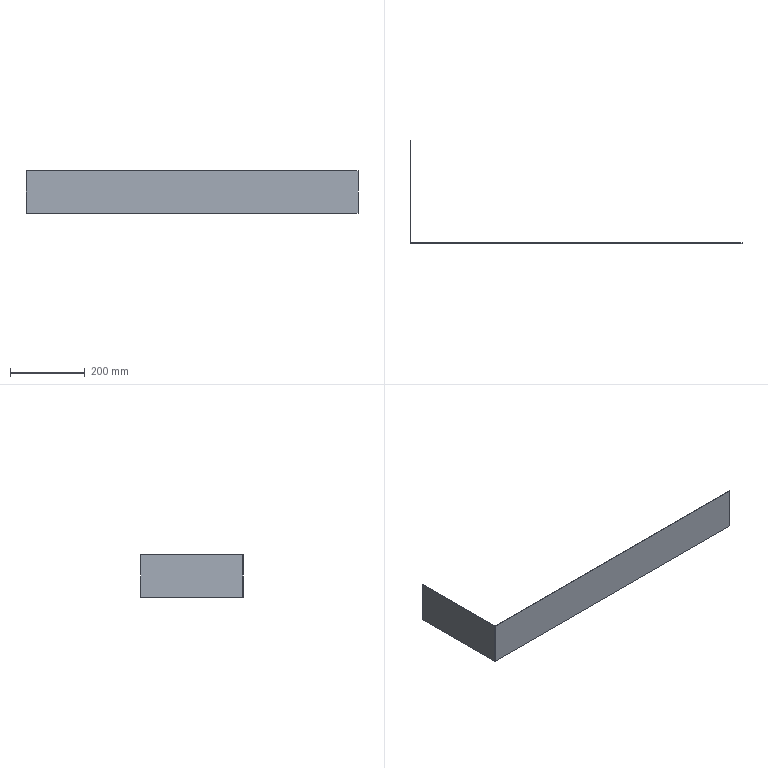Part | STEP file | SX-019-02 | 1 solid | 14 faces | box 890 x 276 x 115 mm | volume 267602 mm3 | plane 12 | cylinder 2 | commonest cylinder face diameters 0.4 x1 4.4 x1
STEP:
#1=CARTESIAN_POINT('',(0.,0.,0.));
#2=DIRECTION('',(0.,0.,1.));
#3=DIRECTION('',(1.,0.,0.));
#4=AXIS2_PLACEMENT_3D('',#1,#2,#3);
#5=CARTESIAN_POINT('',(0.,2.2,115.));
#6=VERTEX_POINT('',#5);
#7=CARTESIAN_POINT('',(2.,2.2,115.));
#8=VERTEX_POINT('',#7);
#9=CARTESIAN_POINT('',(0.,2.2,115.));
#10=DIRECTION('',(1.,0.,0.));
#11=VECTOR('',#10,1.);
#12=LINE('',#9,#11);
#13=CARTESIAN_POINT('',(0.,2.2,115.));
#14=DIRECTION('',(0.,0.,1.));
#15=DIRECTION('',(1.,0.,0.));
#16=AXIS2_PLACEMENT_3D('',#13,#14,#15);
#17=PLANE('',#16);
#18=CARTESIAN_POINT('',(0.,0.));
#19=DIRECTION('',(1.,0.));
#20=VECTOR('',#19,1.);
#21=LINE('',#18,#20);
#22=(GEOMETRIC_REPRESENTATION_CONTEXT(2)PARAMETRIC_REPRESENTATION_CONTEXT()REPRESENTATION_CONTEXT('',''));
#23=DEFINITIONAL_REPRESENTATION('',(#21),#22);
#24=PCURVE('',#17,#23);
#25=CARTESIAN_POINT('',(2.2,2.,115.));
#26=DIRECTION('',(0.,0.,1.));
#27=DIRECTION('',(1.,0.,0.));
#28=AXIS2_PLACEMENT_3D('',#25,#26,#27);
#29=PLANE('',#28);
#30=CARTESIAN_POINT('',(-2.2,0.2));
#31=DIRECTION('',(1.,0.));
#32=VECTOR('',#31,1.);
#33=LINE('',#30,#32);
#34=(GEOMETRIC_REPRESENTATION_CONTEXT(2)PARAMETRIC_REPRESENTATION_CONTEXT()REPRESENTATION_CONTEXT('',''));
#35=DEFINITIONAL_REPRESENTATION('',(#33),#34);
#36=PCURVE('',#29,#35);
#37=SURFACE_CURVE('',#12,(#24,#36),.PCURVE_S1.);
#38=EDGE_CURVE('',#6,#8,#37,.T.);
#39=ORIENTED_EDGE('',*,*,#38,.F.);
#40=CARTESIAN_POINT('',(2.2,0.,115.));
#41=VERTEX_POINT('',#40);
#42=CARTESIAN_POINT('',(2.2,2.2,115.));
#43=DIRECTION('',(0.,0.,1.));
#44=DIRECTION('',(-1.,0.,0.));
#45=AXIS2_PLACEMENT_3D('',#42,#43,#44);
#46=CIRCLE('',#45,2.2);
#47=CARTESIAN_POINT('',(2.2,0.));
#48=DIRECTION('',(-1.,0.));
#49=AXIS2_PLACEMENT_2D('',#47,#48);
#50=CIRCLE('',#49,2.2);
#51=(GEOMETRIC_REPRESENTATION_CONTEXT(2)PARAMETRIC_REPRESENTATION_CONTEXT()REPRESENTATION_CONTEXT('',''));
#52=DEFINITIONAL_REPRESENTATION('',(#50),#51);
#53=PCURVE('',#17,#52);
#54=CARTESIAN_POINT('',(2.2,2.2,115.));
#55=DIRECTION('',(0.,0.,-1.));
#56=DIRECTION('',(-1.,0.,0.));
#57=AXIS2_PLACEMENT_3D('',#54,#55,#56);
#58=CYLINDRICAL_SURFACE('',#57,2.2);
#59=CARTESIAN_POINT('',(6.283,0.));
#60=DIRECTION('',(-1.,0.));
#61=VECTOR('',#60,1.);
#62=LINE('',#59,#61);
#63=(GEOMETRIC_REPRESENTATION_CONTEXT(2)PARAMETRIC_REPRESENTATION_CONTEXT()REPRESENTATION_CONTEXT('',''));
#64=DEFINITIONAL_REPRESENTATION('',(#62),#63);
#65=PCURVE('',#58,#64);
#66=SURFACE_CURVE('',#46,(#53,#65),.PCURVE_S1.);
#67=EDGE_CURVE('',#6,#41,#66,.T.);
#68=ORIENTED_EDGE('',*,*,#67,.T.);
#69=CARTESIAN_POINT('',(2.2,2.,115.));
#70=VERTEX_POINT('',#69);
#71=CARTESIAN_POINT('',(2.2,2.,115.));
#72=DIRECTION('',(0.,-1.,0.));
#73=VECTOR('',#72,1.);
#74=LINE('',#71,#73);
#75=CARTESIAN_POINT('',(2.2,-0.2));
#76=DIRECTION('',(0.,-1.));
#77=VECTOR('',#76,1.);
#78=LINE('',#75,#77);
#79=(GEOMETRIC_REPRESENTATION_CONTEXT(2)PARAMETRIC_REPRESENTATION_CONTEXT()REPRESENTATION_CONTEXT('',''));
#80=DEFINITIONAL_REPRESENTATION('',(#78),#79);
#81=PCURVE('',#17,#80);
#82=CARTESIAN_POINT('',(2.2,2.2,115.));
#83=DIRECTION('',(0.,0.,1.));
#84=DIRECTION('',(1.,0.,0.));
#85=AXIS2_PLACEMENT_3D('',#82,#83,#84);
#86=PLANE('',#85);
#87=CARTESIAN_POINT('',(0.,-0.2));
#88=DIRECTION('',(0.,-1.));
#89=VECTOR('',#88,1.);
#90=LINE('',#87,#89);
#91=(GEOMETRIC_REPRESENTATION_CONTEXT(2)PARAMETRIC_REPRESENTATION_CONTEXT()REPRESENTATION_CONTEXT('',''));
#92=DEFINITIONAL_REPRESENTATION('',(#90),#91);
#93=PCURVE('',#86,#92);
#94=SURFACE_CURVE('',#74,(#81,#93),.PCURVE_S1.);
#95=EDGE_CURVE('',#70,#41,#94,.T.);
#96=ORIENTED_EDGE('',*,*,#95,.F.);
#97=CARTESIAN_POINT('',(2.2,2.2,115.));
#98=DIRECTION('',(0.,0.,1.));
#99=DIRECTION('',(1.,0.,0.));
#100=AXIS2_PLACEMENT_3D('',#97,#98,#99);
#101=CIRCLE('',#100,0.2);
#102=CARTESIAN_POINT('',(2.2,0.));
#103=DIRECTION('',(1.,0.));
#104=AXIS2_PLACEMENT_2D('',#102,#103);
#105=CIRCLE('',#104,0.2);
#106=(GEOMETRIC_REPRESENTATION_CONTEXT(2)PARAMETRIC_REPRESENTATION_CONTEXT()REPRESENTATION_CONTEXT('',''));
#107=DEFINITIONAL_REPRESENTATION('',(#105),#106);
#108=PCURVE('',#17,#107);
#109=CARTESIAN_POINT('',(2.2,2.2,115.));
#110=DIRECTION('',(0.,0.,-1.));
#111=DIRECTION('',(-1.,0.,0.));
#112=AXIS2_PLACEMENT_3D('',#109,#110,#111);
#113=CYLINDRICAL_SURFACE('',#112,0.2);
#114=CARTESIAN_POINT('',(9.425,0.));
#115=DIRECTION('',(-1.,0.));
#116=VECTOR('',#115,1.);
#117=LINE('',#114,#116);
#118=(GEOMETRIC_REPRESENTATION_CONTEXT(2)PARAMETRIC_REPRESENTATION_CONTEXT()REPRESENTATION_CONTEXT('',''));
#119=DEFINITIONAL_REPRESENTATION('',(#117),#118);
#120=PCURVE('',#113,#119);
#121=SURFACE_CURVE('',#101,(#108,#120),.PCURVE_S1.);
#122=EDGE_CURVE('',#8,#70,#121,.T.);
#123=ORIENTED_EDGE('',*,*,#122,.F.);
#124=EDGE_LOOP('',(#39,#68,#96,#123));
#125=FACE_BOUND('',#124,.T.);
#126=ADVANCED_FACE('',(#125),#17,.T.);
#127=CARTESIAN_POINT('',(0.,276.,115.));
#128=VERTEX_POINT('',#127);
#129=CARTESIAN_POINT('',(0.,0.,115.));
#130=DIRECTION('',(0.,-1.,0.));
#131=VECTOR('',#130,1.);
#132=LINE('',#129,#131);
#133=CARTESIAN_POINT('',(-2.2,-2.));
#134=DIRECTION('',(0.,-1.));
#135=VECTOR('',#134,1.);
#136=LINE('',#133,#135);
#137=(GEOMETRIC_REPRESENTATION_CONTEXT(2)PARAMETRIC_REPRESENTATION_CONTEXT()REPRESENTATION_CONTEXT('',''));
#138=DEFINITIONAL_REPRESENTATION('',(#136),#137);
#139=PCURVE('',#29,#138);
#140=CARTESIAN_POINT('',(0.,0.,115.));
#141=DIRECTION('',(1.,0.,0.));
#142=DIRECTION('',(0.,0.,-1.));
#143=AXIS2_PLACEMENT_3D('',#140,#141,#142);
#144=PLANE('',#143);
#145=CARTESIAN_POINT('',(0.,0.));
#146=DIRECTION('',(0.,-1.));
#147=VECTOR('',#146,1.);
#148=LINE('',#145,#147);
#149=(GEOMETRIC_REPRESENTATION_CONTEXT(2)PARAMETRIC_REPRESENTATION_CONTEXT()REPRESENTATION_CONTEXT('',''));
#150=DEFINITIONAL_REPRESENTATION('',(#148),#149);
#151=PCURVE('',#144,#150);
#152=SURFACE_CURVE('',#132,(#139,#151),.PCURVE_S1.);
#153=EDGE_CURVE('',#128,#6,#152,.T.);
#154=ORIENTED_EDGE('',*,*,#153,.T.);
#155=ORIENTED_EDGE('',*,*,#38,.T.);
#156=CARTESIAN_POINT('',(2.,276.,115.));
#157=VERTEX_POINT('',#156);
#158=CARTESIAN_POINT('',(2.,0.,115.));
#159=DIRECTION('',(0.,-1.,0.));
#160=VECTOR('',#159,1.);
#161=LINE('',#158,#160);
#162=CARTESIAN_POINT('',(-0.2,-2.));
#163=DIRECTION('',(0.,-1.));
#164=VECTOR('',#163,1.);
#165=LINE('',#162,#164);
#166=(GEOMETRIC_REPRESENTATION_CONTEXT(2)PARAMETRIC_REPRESENTATION_CONTEXT()REPRESENTATION_CONTEXT('',''));
#167=DEFINITIONAL_REPRESENTATION('',(#165),#166);
#168=PCURVE('',#29,#167);
#169=CARTESIAN_POINT('',(2.,0.,115.));
#170=DIRECTION('',(1.,0.,0.));
#171=DIRECTION('',(0.,0.,-1.));
#172=AXIS2_PLACEMENT_3D('',#169,#170,#171);
#173=PLANE('',#172);
#174=CARTESIAN_POINT('',(0.,0.));
#175=DIRECTION('',(0.,-1.));
#176=VECTOR('',#175,1.);
#177=LINE('',#174,#176);
#178=(GEOMETRIC_REPRESENTATION_CONTEXT(2)PARAMETRIC_REPRESENTATION_CONTEXT()REPRESENTATION_CONTEXT('',''));
#179=DEFINITIONAL_REPRESENTATION('',(#177),#178);
#180=PCURVE('',#173,#179);
#181=SURFACE_CURVE('',#161,(#168,#180),.PCURVE_S1.);
#182=EDGE_CURVE('',#157,#8,#181,.T.);
#183=ORIENTED_EDGE('',*,*,#182,.F.);
#184=CARTESIAN_POINT('',(0.,276.,115.));
#185=DIRECTION('',(1.,0.,0.));
#186=VECTOR('',#185,1.);
#187=LINE('',#184,#186);
#188=CARTESIAN_POINT('',(-2.2,274.));
#189=DIRECTION('',(1.,0.));
#190=VECTOR('',#189,1.);
#191=LINE('',#188,#190);
#192=(GEOMETRIC_REPRESENTATION_CONTEXT(2)PARAMETRIC_REPRESENTATION_CONTEXT()REPRESENTATION_CONTEXT('',''));
#193=DEFINITIONAL_REPRESENTATION('',(#191),#192);
#194=PCURVE('',#29,#193);
#195=CARTESIAN_POINT('',(0.,276.,115.));
#196=DIRECTION('',(0.,1.,0.));
#197=DIRECTION('',(0.,0.,1.));
#198=AXIS2_PLACEMENT_3D('',#195,#196,#197);
#199=PLANE('',#198);
#200=CARTESIAN_POINT('',(0.,0.));
#201=DIRECTION('',(0.,1.));
#202=VECTOR('',#201,1.);
#203=LINE('',#200,#202);
#204=(GEOMETRIC_REPRESENTATION_CONTEXT(2)PARAMETRIC_REPRESENTATION_CONTEXT()REPRESENTATION_CONTEXT('',''));
#205=DEFINITIONAL_REPRESENTATION('',(#203),#204);
#206=PCURVE('',#199,#205);
#207=SURFACE_CURVE('',#187,(#194,#206),.PCURVE_S1.);
#208=EDGE_CURVE('',#128,#157,#207,.T.);
#209=ORIENTED_EDGE('',*,*,#208,.F.);
#210=EDGE_LOOP('',(#154,#155,#183,#209));
#211=FACE_BOUND('',#210,.T.);
#212=ADVANCED_FACE('',(#211),#29,.T.);
#213=CARTESIAN_POINT('',(2.2,0.,0.));
#214=VERTEX_POINT('',#213);
#215=CARTESIAN_POINT('',(2.2,2.,0.));
#216=VERTEX_POINT('',#215);
#217=CARTESIAN_POINT('',(2.2,0.,0.));
#218=DIRECTION('',(0.,1.,0.));
#219=VECTOR('',#218,1.);
#220=LINE('',#217,#219);
#221=CARTESIAN_POINT('',(2.2,0.,0.));
#222=DIRECTION('',(0.,0.,-1.));
#223=DIRECTION('',(-1.,0.,0.));
#224=AXIS2_PLACEMENT_3D('',#221,#222,#223);
#225=PLANE('',#224);
#226=CARTESIAN_POINT('',(0.,0.));
#227=DIRECTION('',(0.,1.));
#228=VECTOR('',#227,1.);
#229=LINE('',#226,#228);
#230=(GEOMETRIC_REPRESENTATION_CONTEXT(2)PARAMETRIC_REPRESENTATION_CONTEXT()REPRESENTATION_CONTEXT('',''));
#231=DEFINITIONAL_REPRESENTATION('',(#229),#230);
#232=PCURVE('',#225,#231);
#233=CARTESIAN_POINT('',(2.,2.2,0.));
#234=DIRECTION('',(0.,0.,-1.));
#235=DIRECTION('',(-1.,0.,0.));
#236=AXIS2_PLACEMENT_3D('',#233,#234,#235);
#237=PLANE('',#236);
#238=CARTESIAN_POINT('',(-0.2,-2.2));
#239=DIRECTION('',(0.,1.));
#240=VECTOR('',#239,1.);
#241=LINE('',#238,#240);
#242=(GEOMETRIC_REPRESENTATION_CONTEXT(2)PARAMETRIC_REPRESENTATION_CONTEXT()REPRESENTATION_CONTEXT('',''));
#243=DEFINITIONAL_REPRESENTATION('',(#241),#242);
#244=PCURVE('',#237,#243);
#245=SURFACE_CURVE('',#220,(#232,#244),.PCURVE_S1.);
#246=EDGE_CURVE('',#214,#216,#245,.T.);
#247=ORIENTED_EDGE('',*,*,#246,.F.);
#248=CARTESIAN_POINT('',(0.,2.2,0.));
#249=VERTEX_POINT('',#248);
#250=CARTESIAN_POINT('',(2.2,2.2,0.));
#251=DIRECTION('',(0.,0.,1.));
#252=DIRECTION('',(-1.,0.,0.));
#253=AXIS2_PLACEMENT_3D('',#250,#251,#252);
#254=CIRCLE('',#253,2.2);
#255=CARTESIAN_POINT('',(2.2,2.2));
#256=CARTESIAN_POINT('',(2.2,-1.611));
#257=CARTESIAN_POINT('',(-1.1,0.2947));
#258=CARTESIAN_POINT('',(-4.4,2.2));
#259=CARTESIAN_POINT('',(-1.1,4.105));
#260=CARTESIAN_POINT('',(2.2,6.011));
#261=CARTESIAN_POINT('',(2.2,2.2));
#262=(BOUNDED_CURVE()B_SPLINE_CURVE(2,(#255,#256,#257,#258,#259,#260,#261),.UNSPECIFIED.,.T.,.F.)B_SPLINE_CURVE_WITH_KNOTS((1,2,2,2,2,1),(-2.094,0.,2.094,4.189,6.283,8.378),.UNSPECIFIED.)CURVE()GEOMETRIC_REPRESENTATION_ITEM()RATIONAL_B_SPLINE_CURVE((1.,0.5,1.,0.5,1.,0.5,1.))REPRESENTATION_ITEM(''));
#263=(GEOMETRIC_REPRESENTATION_CONTEXT(2)PARAMETRIC_REPRESENTATION_CONTEXT()REPRESENTATION_CONTEXT('',''));
#264=DEFINITIONAL_REPRESENTATION('',(#262),#263);
#265=PCURVE('',#225,#264);
#266=CARTESIAN_POINT('',(6.283,115.));
#267=DIRECTION('',(-1.,0.));
#268=VECTOR('',#267,1.);
#269=LINE('',#266,#268);
#270=(GEOMETRIC_REPRESENTATION_CONTEXT(2)PARAMETRIC_REPRESENTATION_CONTEXT()REPRESENTATION_CONTEXT('',''));
#271=DEFINITIONAL_REPRESENTATION('',(#269),#270);
#272=PCURVE('',#58,#271);
#273=SURFACE_CURVE('',#254,(#265,#272),.PCURVE_S1.);
#274=EDGE_CURVE('',#249,#214,#273,.T.);
#275=ORIENTED_EDGE('',*,*,#274,.F.);
#276=CARTESIAN_POINT('',(2.,2.2,0.));
#277=VERTEX_POINT('',#276);
#278=CARTESIAN_POINT('',(2.,2.2,0.));
#279=DIRECTION('',(-1.,0.,0.));
#280=VECTOR('',#279,1.);
#281=LINE('',#278,#280);
#282=CARTESIAN_POINT('',(0.2,2.2));
#283=DIRECTION('',(1.,0.));
#284=VECTOR('',#283,1.);
#285=LINE('',#282,#284);
#286=(GEOMETRIC_REPRESENTATION_CONTEXT(2)PARAMETRIC_REPRESENTATION_CONTEXT()REPRESENTATION_CONTEXT('',''));
#287=DEFINITIONAL_REPRESENTATION('',(#285),#286);
#288=PCURVE('',#225,#287);
#289=CARTESIAN_POINT('',(2.2,2.2,0.));
#290=DIRECTION('',(0.,0.,1.));
#291=DIRECTION('',(1.,0.,0.));
#292=AXIS2_PLACEMENT_3D('',#289,#290,#291);
#293=PLANE('',#292);
#294=CARTESIAN_POINT('',(-0.2,0.));
#295=DIRECTION('',(-1.,0.));
#296=VECTOR('',#295,1.);
#297=LINE('',#294,#296);
#298=(GEOMETRIC_REPRESENTATION_CONTEXT(2)PARAMETRIC_REPRESENTATION_CONTEXT()REPRESENTATION_CONTEXT('',''));
#299=DEFINITIONAL_REPRESENTATION('',(#297),#298);
#300=PCURVE('',#293,#299);
#301=SURFACE_CURVE('',#281,(#288,#300),.PCURVE_S1.);
#302=EDGE_CURVE('',#277,#249,#301,.T.);
#303=ORIENTED_EDGE('',*,*,#302,.F.);
#304=CARTESIAN_POINT('',(2.2,2.2,0.));
#305=DIRECTION('',(0.,0.,1.));
#306=DIRECTION('',(1.,0.,0.));
#307=AXIS2_PLACEMENT_3D('',#304,#305,#306);
#308=CIRCLE('',#307,0.2);
#309=CARTESIAN_POINT('',(-0.2,2.2));
#310=CARTESIAN_POINT('',(-0.2,2.546));
#311=CARTESIAN_POINT('',(0.1,2.373));
#312=CARTESIAN_POINT('',(0.4,2.2));
#313=CARTESIAN_POINT('',(0.1,2.027));
#314=CARTESIAN_POINT('',(-0.2,1.854));
#315=CARTESIAN_POINT('',(-0.2,2.2));
#316=(BOUNDED_CURVE()B_SPLINE_CURVE(2,(#309,#310,#311,#312,#313,#314,#315),.UNSPECIFIED.,.T.,.F.)B_SPLINE_CURVE_WITH_KNOTS((1,2,2,2,2,1),(-2.094,0.,2.094,4.189,6.283,8.378),.UNSPECIFIED.)CURVE()GEOMETRIC_REPRESENTATION_ITEM()RATIONAL_B_SPLINE_CURVE((1.,0.5,1.,0.5,1.,0.5,1.))REPRESENTATION_ITEM(''));
#317=(GEOMETRIC_REPRESENTATION_CONTEXT(2)PARAMETRIC_REPRESENTATION_CONTEXT()REPRESENTATION_CONTEXT('',''));
#318=DEFINITIONAL_REPRESENTATION('',(#316),#317);
#319=PCURVE('',#225,#318);
#320=CARTESIAN_POINT('',(9.425,115.));
#321=DIRECTION('',(-1.,0.));
#322=VECTOR('',#321,1.);
#323=LINE('',#320,#322);
#324=(GEOMETRIC_REPRESENTATION_CONTEXT(2)PARAMETRIC_REPRESENTATION_CONTEXT()REPRESENTATION_CONTEXT('',''));
#325=DEFINITIONAL_REPRESENTATION('',(#323),#324);
#326=PCURVE('',#113,#325);
#327=SURFACE_CURVE('',#308,(#319,#326),.PCURVE_S1.);
#328=EDGE_CURVE('',#277,#216,#327,.T.);
#329=ORIENTED_EDGE('',*,*,#328,.T.);
#330=EDGE_LOOP('',(#247,#275,#303,#329));
#331=FACE_BOUND('',#330,.T.);
#332=ADVANCED_FACE('',(#331),#225,.T.);
#333=CARTESIAN_POINT('',(890.,0.,0.));
#334=VERTEX_POINT('',#333);
#335=CARTESIAN_POINT('',(0.,0.,0.));
#336=DIRECTION('',(1.,0.,0.));
#337=VECTOR('',#336,1.);
#338=LINE('',#335,#337);
#339=CARTESIAN_POINT('',(2.,-2.2));
#340=DIRECTION('',(-1.,0.));
#341=VECTOR('',#340,1.);
#342=LINE('',#339,#341);
#343=(GEOMETRIC_REPRESENTATION_CONTEXT(2)PARAMETRIC_REPRESENTATION_CONTEXT()REPRESENTATION_CONTEXT('',''));
#344=DEFINITIONAL_REPRESENTATION('',(#342),#343);
#345=PCURVE('',#237,#344);
#346=CARTESIAN_POINT('',(0.,0.,115.));
#347=DIRECTION('',(0.,1.,0.));
#348=DIRECTION('',(0.,0.,1.));
#349=AXIS2_PLACEMENT_3D('',#346,#347,#348);
#350=PLANE('',#349);
#351=CARTESIAN_POINT('',(-115.,0.));
#352=DIRECTION('',(0.,1.));
#353=VECTOR('',#352,1.);
#354=LINE('',#351,#353);
#355=(GEOMETRIC_REPRESENTATION_CONTEXT(2)PARAMETRIC_REPRESENTATION_CONTEXT()REPRESENTATION_CONTEXT('',''));
#356=DEFINITIONAL_REPRESENTATION('',(#354),#355);
#357=PCURVE('',#350,#356);
#358=SURFACE_CURVE('',#338,(#345,#357),.PCURVE_S1.);
#359=EDGE_CURVE('',#214,#334,#358,.T.);
#360=ORIENTED_EDGE('',*,*,#359,.F.);
#361=ORIENTED_EDGE('',*,*,#246,.T.);
#362=CARTESIAN_POINT('',(890.,2.,0.));
#363=VERTEX_POINT('',#362);
#364=CARTESIAN_POINT('',(0.,2.,0.));
#365=DIRECTION('',(1.,0.,0.));
#366=VECTOR('',#365,1.);
#367=LINE('',#364,#366);
#368=CARTESIAN_POINT('',(2.,-0.2));
#369=DIRECTION('',(-1.,0.));
#370=VECTOR('',#369,1.);
#371=LINE('',#368,#370);
#372=(GEOMETRIC_REPRESENTATION_CONTEXT(2)PARAMETRIC_REPRESENTATION_CONTEXT()REPRESENTATION_CONTEXT('',''));
#373=DEFINITIONAL_REPRESENTATION('',(#371),#372);
#374=PCURVE('',#237,#373);
#375=CARTESIAN_POINT('',(0.,2.,115.));
#376=DIRECTION('',(0.,1.,0.));
#377=DIRECTION('',(0.,0.,1.));
#378=AXIS2_PLACEMENT_3D('',#375,#376,#377);
#379=PLANE('',#378);
#380=CARTESIAN_POINT('',(-115.,0.));
#381=DIRECTION('',(0.,1.));
#382=VECTOR('',#381,1.);
#383=LINE('',#380,#382);
#384=(GEOMETRIC_REPRESENTATION_CONTEXT(2)PARAMETRIC_REPRESENTATION_CONTEXT()REPRESENTATION_CONTEXT('',''));
#385=DEFINITIONAL_REPRESENTATION('',(#383),#384);
#386=PCURVE('',#379,#385);
#387=SURFACE_CURVE('',#367,(#374,#386),.PCURVE_S1.);
#388=EDGE_CURVE('',#216,#363,#387,.T.);
#389=ORIENTED_EDGE('',*,*,#388,.T.);
#390=CARTESIAN_POINT('',(890.,2.,0.));
#391=DIRECTION('',(0.,-1.,0.));
#392=VECTOR('',#391,1.);
#393=LINE('',#390,#392);
#394=CARTESIAN_POINT('',(-888.,-0.2));
#395=DIRECTION('',(0.,-1.));
#396=VECTOR('',#395,1.);
#397=LINE('',#394,#396);
#398=(GEOMETRIC_REPRESENTATION_CONTEXT(2)PARAMETRIC_REPRESENTATION_CONTEXT()REPRESENTATION_CONTEXT('',''));
#399=DEFINITIONAL_REPRESENTATION('',(#397),#398);
#400=PCURVE('',#237,#399);
#401=CARTESIAN_POINT('',(890.,2.,115.));
#402=DIRECTION('',(1.,0.,0.));
#403=DIRECTION('',(0.,0.,-1.));
#404=AXIS2_PLACEMENT_3D('',#401,#402,#403);
#405=PLANE('',#404);
#406=CARTESIAN_POINT('',(115.,0.));
#407=DIRECTION('',(0.,-1.));
#408=VECTOR('',#407,1.);
#409=LINE('',#406,#408);
#410=(GEOMETRIC_REPRESENTATION_CONTEXT(2)PARAMETRIC_REPRESENTATION_CONTEXT()REPRESENTATION_CONTEXT('',''));
#411=DEFINITIONAL_REPRESENTATION('',(#409),#410);
#412=PCURVE('',#405,#411);
#413=SURFACE_CURVE('',#393,(#400,#412),.PCURVE_S1.);
#414=EDGE_CURVE('',#363,#334,#413,.T.);
#415=ORIENTED_EDGE('',*,*,#414,.T.);
#416=EDGE_LOOP('',(#360,#361,#389,#415));
#417=FACE_BOUND('',#416,.T.);
#418=ADVANCED_FACE('',(#417),#237,.T.);
#419=ORIENTED_EDGE('',*,*,#359,.T.);
#420=CARTESIAN_POINT('',(890.,0.,115.));
#421=VERTEX_POINT('',#420);
#422=CARTESIAN_POINT('',(890.,0.,115.));
#423=DIRECTION('',(0.,0.,-1.));
#424=VECTOR('',#423,1.);
#425=LINE('',#422,#424);
#426=CARTESIAN_POINT('',(0.,890.));
#427=DIRECTION('',(-1.,0.));
#428=VECTOR('',#427,1.);
#429=LINE('',#426,#428);
#430=(GEOMETRIC_REPRESENTATION_CONTEXT(2)PARAMETRIC_REPRESENTATION_CONTEXT()REPRESENTATION_CONTEXT('',''));
#431=DEFINITIONAL_REPRESENTATION('',(#429),#430);
#432=PCURVE('',#350,#431);
#433=CARTESIAN_POINT('',(0.,-2.));
#434=DIRECTION('',(1.,0.));
#435=VECTOR('',#434,1.);
#436=LINE('',#433,#435);
#437=(GEOMETRIC_REPRESENTATION_CONTEXT(2)PARAMETRIC_REPRESENTATION_CONTEXT()REPRESENTATION_CONTEXT('',''));
#438=DEFINITIONAL_REPRESENTATION('',(#436),#437);
#439=PCURVE('',#405,#438);
#440=SURFACE_CURVE('',#425,(#432,#439),.PCURVE_S1.);
#441=EDGE_CURVE('',#421,#334,#440,.T.);
#442=ORIENTED_EDGE('',*,*,#441,.F.);
#443=CARTESIAN_POINT('',(0.,0.,115.));
#444=DIRECTION('',(1.,0.,0.));
#445=VECTOR('',#444,1.);
#446=LINE('',#443,#445);
#447=CARTESIAN_POINT('',(0.,0.));
#448=DIRECTION('',(0.,1.));
#449=VECTOR('',#448,1.);
#450=LINE('',#447,#449);
#451=(GEOMETRIC_REPRESENTATION_CONTEXT(2)PARAMETRIC_REPRESENTATION_CONTEXT()REPRESENTATION_CONTEXT('',''));
#452=DEFINITIONAL_REPRESENTATION('',(#450),#451);
#453=PCURVE('',#350,#452);
#454=CARTESIAN_POINT('',(-2.2,-2.2));
#455=DIRECTION('',(1.,0.));
#456=VECTOR('',#455,1.);
#457=LINE('',#454,#456);
#458=(GEOMETRIC_REPRESENTATION_CONTEXT(2)PARAMETRIC_REPRESENTATION_CONTEXT()REPRESENTATION_CONTEXT('',''));
#459=DEFINITIONAL_REPRESENTATION('',(#457),#458);
#460=PCURVE('',#86,#459);
#461=SURFACE_CURVE('',#446,(#453,#460),.PCURVE_S1.);
#462=EDGE_CURVE('',#41,#421,#461,.T.);
#463=ORIENTED_EDGE('',*,*,#462,.F.);
#464=CARTESIAN_POINT('',(2.2,0.,115.));
#465=DIRECTION('',(0.,0.,-1.));
#466=VECTOR('',#465,1.);
#467=LINE('',#464,#466);
#468=CARTESIAN_POINT('',(0.,2.2));
#469=DIRECTION('',(-1.,0.));
#470=VECTOR('',#469,1.);
#471=LINE('',#468,#470);
#472=(GEOMETRIC_REPRESENTATION_CONTEXT(2)PARAMETRIC_REPRESENTATION_CONTEXT()REPRESENTATION_CONTEXT('',''));
#473=DEFINITIONAL_REPRESENTATION('',(#471),#472);
#474=PCURVE('',#350,#473);
#475=CARTESIAN_POINT('',(4.712,0.));
#476=DIRECTION('',(0.,1.));
#477=VECTOR('',#476,1.);
#478=LINE('',#475,#477);
#479=(GEOMETRIC_REPRESENTATION_CONTEXT(2)PARAMETRIC_REPRESENTATION_CONTEXT()REPRESENTATION_CONTEXT('',''));
#480=DEFINITIONAL_REPRESENTATION('',(#478),#479);
#481=PCURVE('',#58,#480);
#482=SURFACE_CURVE('',#467,(#474,#481),.PCURVE_S1.);
#483=EDGE_CURVE('',#41,#214,#482,.T.);
#484=ORIENTED_EDGE('',*,*,#483,.T.);
#485=EDGE_LOOP('',(#419,#442,#463,#484));
#486=FACE_BOUND('',#485,.T.);
#487=ADVANCED_FACE('',(#486),#350,.F.);
#488=ORIENTED_EDGE('',*,*,#414,.F.);
#489=CARTESIAN_POINT('',(890.,2.,115.));
#490=VERTEX_POINT('',#489);
#491=CARTESIAN_POINT('',(890.,2.,115.));
#492=DIRECTION('',(0.,0.,-1.));
#493=VECTOR('',#492,1.);
#494=LINE('',#491,#493);
#495=CARTESIAN_POINT('',(0.,0.));
#496=DIRECTION('',(1.,0.));
#497=VECTOR('',#496,1.);
#498=LINE('',#495,#497);
#499=(GEOMETRIC_REPRESENTATION_CONTEXT(2)PARAMETRIC_REPRESENTATION_CONTEXT()REPRESENTATION_CONTEXT('',''));
#500=DEFINITIONAL_REPRESENTATION('',(#498),#499);
#501=PCURVE('',#405,#500);
#502=CARTESIAN_POINT('',(0.,890.));
#503=DIRECTION('',(-1.,0.));
#504=VECTOR('',#503,1.);
#505=LINE('',#502,#504);
#506=(GEOMETRIC_REPRESENTATION_CONTEXT(2)PARAMETRIC_REPRESENTATION_CONTEXT()REPRESENTATION_CONTEXT('',''));
#507=DEFINITIONAL_REPRESENTATION('',(#505),#506);
#508=PCURVE('',#379,#507);
#509=SURFACE_CURVE('',#494,(#501,#508),.PCURVE_S1.);
#510=EDGE_CURVE('',#490,#363,#509,.T.);
#511=ORIENTED_EDGE('',*,*,#510,.F.);
#512=CARTESIAN_POINT('',(890.,2.,115.));
#513=DIRECTION('',(0.,-1.,0.));
#514=VECTOR('',#513,1.);
#515=LINE('',#512,#514);
#516=CARTESIAN_POINT('',(0.,0.));
#517=DIRECTION('',(0.,-1.));
#518=VECTOR('',#517,1.);
#519=LINE('',#516,#518);
#520=(GEOMETRIC_REPRESENTATION_CONTEXT(2)PARAMETRIC_REPRESENTATION_CONTEXT()REPRESENTATION_CONTEXT('',''));
#521=DEFINITIONAL_REPRESENTATION('',(#519),#520);
#522=PCURVE('',#405,#521);
#523=CARTESIAN_POINT('',(887.8,-0.2));
#524=DIRECTION('',(0.,-1.));
#525=VECTOR('',#524,1.);
#526=LINE('',#523,#525);
#527=(GEOMETRIC_REPRESENTATION_CONTEXT(2)PARAMETRIC_REPRESENTATION_CONTEXT()REPRESENTATION_CONTEXT('',''));
#528=DEFINITIONAL_REPRESENTATION('',(#526),#527);
#529=PCURVE('',#86,#528);
#530=SURFACE_CURVE('',#515,(#522,#529),.PCURVE_S1.);
#531=EDGE_CURVE('',#490,#421,#530,.T.);
#532=ORIENTED_EDGE('',*,*,#531,.T.);
#533=ORIENTED_EDGE('',*,*,#441,.T.);
#534=EDGE_LOOP('',(#488,#511,#532,#533));
#535=FACE_BOUND('',#534,.T.);
#536=ADVANCED_FACE('',(#535),#405,.T.);
#537=ORIENTED_EDGE('',*,*,#388,.F.);
#538=CARTESIAN_POINT('',(2.2,2.,115.));
#539=DIRECTION('',(0.,0.,-1.));
#540=VECTOR('',#539,1.);
#541=LINE('',#538,#540);
#542=CARTESIAN_POINT('',(0.,2.2));
#543=DIRECTION('',(-1.,0.));
#544=VECTOR('',#543,1.);
#545=LINE('',#542,#544);
#546=(GEOMETRIC_REPRESENTATION_CONTEXT(2)PARAMETRIC_REPRESENTATION_CONTEXT()REPRESENTATION_CONTEXT('',''));
#547=DEFINITIONAL_REPRESENTATION('',(#545),#546);
#548=PCURVE('',#379,#547);
#549=CARTESIAN_POINT('',(4.712,0.));
#550=DIRECTION('',(0.,1.));
#551=VECTOR('',#550,1.);
#552=LINE('',#549,#551);
#553=(GEOMETRIC_REPRESENTATION_CONTEXT(2)PARAMETRIC_REPRESENTATION_CONTEXT()REPRESENTATION_CONTEXT('',''));
#554=DEFINITIONAL_REPRESENTATION('',(#552),#553);
#555=PCURVE('',#113,#554);
#556=SURFACE_CURVE('',#541,(#548,#555),.PCURVE_S1.);
#557=EDGE_CURVE('',#70,#216,#556,.T.);
#558=ORIENTED_EDGE('',*,*,#557,.F.);
#559=CARTESIAN_POINT('',(0.,2.,115.));
#560=DIRECTION('',(1.,0.,0.));
#561=VECTOR('',#560,1.);
#562=LINE('',#559,#561);
#563=CARTESIAN_POINT('',(0.,0.));
#564=DIRECTION('',(0.,1.));
#565=VECTOR('',#564,1.);
#566=LINE('',#563,#565);
#567=(GEOMETRIC_REPRESENTATION_CONTEXT(2)PARAMETRIC_REPRESENTATION_CONTEXT()REPRESENTATION_CONTEXT('',''));
#568=DEFINITIONAL_REPRESENTATION('',(#566),#567);
#569=PCURVE('',#379,#568);
#570=CARTESIAN_POINT('',(-2.2,-0.2));
#571=DIRECTION('',(1.,0.));
#572=VECTOR('',#571,1.);
#573=LINE('',#570,#572);
#574=(GEOMETRIC_REPRESENTATION_CONTEXT(2)PARAMETRIC_REPRESENTATION_CONTEXT()REPRESENTATION_CONTEXT('',''));
#575=DEFINITIONAL_REPRESENTATION('',(#573),#574);
#576=PCURVE('',#86,#575);
#577=SURFACE_CURVE('',#562,(#569,#576),.PCURVE_S1.);
#578=EDGE_CURVE('',#70,#490,#577,.T.);
#579=ORIENTED_EDGE('',*,*,#578,.T.);
#580=ORIENTED_EDGE('',*,*,#510,.T.);
#581=EDGE_LOOP('',(#537,#558,#579,#580));
#582=FACE_BOUND('',#581,.T.);
#583=ADVANCED_FACE('',(#582),#379,.T.);
#584=ORIENTED_EDGE('',*,*,#557,.F.);
#585=ORIENTED_EDGE('',*,*,#122,.F.);
#586=CARTESIAN_POINT('',(2.,2.2,115.));
#587=DIRECTION('',(0.,0.,-1.));
#588=VECTOR('',#587,1.);
#589=LINE('',#586,#588);
#590=CARTESIAN_POINT('',(6.283,0.));
#591=DIRECTION('',(0.,1.));
#592=VECTOR('',#591,1.);
#593=LINE('',#590,#592);
#594=(GEOMETRIC_REPRESENTATION_CONTEXT(2)PARAMETRIC_REPRESENTATION_CONTEXT()REPRESENTATION_CONTEXT('',''));
#595=DEFINITIONAL_REPRESENTATION('',(#593),#594);
#596=PCURVE('',#113,#595);
#597=CARTESIAN_POINT('',(0.,2.2));
#598=DIRECTION('',(1.,0.));
#599=VECTOR('',#598,1.);
#600=LINE('',#597,#599);
#601=(GEOMETRIC_REPRESENTATION_CONTEXT(2)PARAMETRIC_REPRESENTATION_CONTEXT()REPRESENTATION_CONTEXT('',''));
#602=DEFINITIONAL_REPRESENTATION('',(#600),#601);
#603=PCURVE('',#173,#602);
#604=SURFACE_CURVE('',#589,(#596,#603),.PCURVE_S1.);
#605=EDGE_CURVE('',#8,#277,#604,.T.);
#606=ORIENTED_EDGE('',*,*,#605,.T.);
#607=ORIENTED_EDGE('',*,*,#328,.T.);
#608=EDGE_LOOP('',(#584,#585,#606,#607));
#609=FACE_BOUND('',#608,.F.);
#610=ADVANCED_FACE('',(#609),#113,.F.);
#611=CARTESIAN_POINT('',(2.,276.,0.));
#612=VERTEX_POINT('',#611);
#613=CARTESIAN_POINT('',(2.,0.,0.));
#614=DIRECTION('',(0.,-1.,0.));
#615=VECTOR('',#614,1.);
#616=LINE('',#613,#615);
#617=CARTESIAN_POINT('',(115.,0.));
#618=DIRECTION('',(0.,-1.));
#619=VECTOR('',#618,1.);
#620=LINE('',#617,#619);
#621=(GEOMETRIC_REPRESENTATION_CONTEXT(2)PARAMETRIC_REPRESENTATION_CONTEXT()REPRESENTATION_CONTEXT('',''));
#622=DEFINITIONAL_REPRESENTATION('',(#620),#621);
#623=PCURVE('',#173,#622);
#624=CARTESIAN_POINT('',(-0.2,-2.2));
#625=DIRECTION('',(0.,-1.));
#626=VECTOR('',#625,1.);
#627=LINE('',#624,#626);
#628=(GEOMETRIC_REPRESENTATION_CONTEXT(2)PARAMETRIC_REPRESENTATION_CONTEXT()REPRESENTATION_CONTEXT('',''));
#629=DEFINITIONAL_REPRESENTATION('',(#627),#628);
#630=PCURVE('',#293,#629);
#631=SURFACE_CURVE('',#616,(#623,#630),.PCURVE_S1.);
#632=EDGE_CURVE('',#612,#277,#631,.T.);
#633=ORIENTED_EDGE('',*,*,#632,.F.);
#634=CARTESIAN_POINT('',(2.,276.,115.));
#635=DIRECTION('',(0.,0.,-1.));
#636=VECTOR('',#635,1.);
#637=LINE('',#634,#636);
#638=CARTESIAN_POINT('',(0.,276.));
#639=DIRECTION('',(1.,0.));
#640=VECTOR('',#639,1.);
#641=LINE('',#638,#640);
#642=(GEOMETRIC_REPRESENTATION_CONTEXT(2)PARAMETRIC_REPRESENTATION_CONTEXT()REPRESENTATION_CONTEXT('',''));
#643=DEFINITIONAL_REPRESENTATION('',(#641),#642);
#644=PCURVE('',#173,#643);
#645=CARTESIAN_POINT('',(0.,2.));
#646=DIRECTION('',(-1.,0.));
#647=VECTOR('',#646,1.);
#648=LINE('',#645,#647);
#649=(GEOMETRIC_REPRESENTATION_CONTEXT(2)PARAMETRIC_REPRESENTATION_CONTEXT()REPRESENTATION_CONTEXT('',''));
#650=DEFINITIONAL_REPRESENTATION('',(#648),#649);
#651=PCURVE('',#199,#650);
#652=SURFACE_CURVE('',#637,(#644,#651),.PCURVE_S1.);
#653=EDGE_CURVE('',#157,#612,#652,.T.);
#654=ORIENTED_EDGE('',*,*,#653,.F.);
#655=ORIENTED_EDGE('',*,*,#182,.T.);
#656=ORIENTED_EDGE('',*,*,#605,.T.);
#657=EDGE_LOOP('',(#633,#654,#655,#656));
#658=FACE_BOUND('',#657,.T.);
#659=ADVANCED_FACE('',(#658),#173,.T.);
#660=CARTESIAN_POINT('',(0.,276.,0.));
#661=VERTEX_POINT('',#660);
#662=CARTESIAN_POINT('',(0.,276.,0.));
#663=DIRECTION('',(1.,0.,0.));
#664=VECTOR('',#663,1.);
#665=LINE('',#662,#664);
#666=CARTESIAN_POINT('',(-115.,0.));
#667=DIRECTION('',(0.,1.));
#668=VECTOR('',#667,1.);
#669=LINE('',#666,#668);
#670=(GEOMETRIC_REPRESENTATION_CONTEXT(2)PARAMETRIC_REPRESENTATION_CONTEXT()REPRESENTATION_CONTEXT('',''));
#671=DEFINITIONAL_REPRESENTATION('',(#669),#670);
#672=PCURVE('',#199,#671);
#673=CARTESIAN_POINT('',(-2.2,273.8));
#674=DIRECTION('',(1.,0.));
#675=VECTOR('',#674,1.);
#676=LINE('',#673,#675);
#677=(GEOMETRIC_REPRESENTATION_CONTEXT(2)PARAMETRIC_REPRESENTATION_CONTEXT()REPRESENTATION_CONTEXT('',''));
#678=DEFINITIONAL_REPRESENTATION('',(#676),#677);
#679=PCURVE('',#293,#678);
#680=SURFACE_CURVE('',#665,(#672,#679),.PCURVE_S1.);
#681=EDGE_CURVE('',#661,#612,#680,.T.);
#682=ORIENTED_EDGE('',*,*,#681,.F.);
#683=CARTESIAN_POINT('',(0.,276.,115.));
#684=DIRECTION('',(0.,0.,-1.));
#685=VECTOR('',#684,1.);
#686=LINE('',#683,#685);
#687=CARTESIAN_POINT('',(0.,0.));
#688=DIRECTION('',(-1.,0.));
#689=VECTOR('',#688,1.);
#690=LINE('',#687,#689);
#691=(GEOMETRIC_REPRESENTATION_CONTEXT(2)PARAMETRIC_REPRESENTATION_CONTEXT()REPRESENTATION_CONTEXT('',''));
#692=DEFINITIONAL_REPRESENTATION('',(#690),#691);
#693=PCURVE('',#199,#692);
#694=CARTESIAN_POINT('',(0.,276.));
#695=DIRECTION('',(1.,0.));
#696=VECTOR('',#695,1.);
#697=LINE('',#694,#696);
#698=(GEOMETRIC_REPRESENTATION_CONTEXT(2)PARAMETRIC_REPRESENTATION_CONTEXT()REPRESENTATION_CONTEXT('',''));
#699=DEFINITIONAL_REPRESENTATION('',(#697),#698);
#700=PCURVE('',#144,#699);
#701=SURFACE_CURVE('',#686,(#693,#700),.PCURVE_S1.);
#702=EDGE_CURVE('',#128,#661,#701,.T.);
#703=ORIENTED_EDGE('',*,*,#702,.F.);
#704=ORIENTED_EDGE('',*,*,#208,.T.);
#705=ORIENTED_EDGE('',*,*,#653,.T.);
#706=EDGE_LOOP('',(#682,#703,#704,#705));
#707=FACE_BOUND('',#706,.T.);
#708=ADVANCED_FACE('',(#707),#199,.T.);
#709=CARTESIAN_POINT('',(0.,0.,0.));
#710=DIRECTION('',(0.,-1.,0.));
#711=VECTOR('',#710,1.);
#712=LINE('',#709,#711);
#713=CARTESIAN_POINT('',(115.,0.));
#714=DIRECTION('',(0.,-1.));
#715=VECTOR('',#714,1.);
#716=LINE('',#713,#715);
#717=(GEOMETRIC_REPRESENTATION_CONTEXT(2)PARAMETRIC_REPRESENTATION_CONTEXT()REPRESENTATION_CONTEXT('',''));
#718=DEFINITIONAL_REPRESENTATION('',(#716),#717);
#719=PCURVE('',#144,#718);
#720=CARTESIAN_POINT('',(-2.2,-2.2));
#721=DIRECTION('',(0.,-1.));
#722=VECTOR('',#721,1.);
#723=LINE('',#720,#722);
#724=(GEOMETRIC_REPRESENTATION_CONTEXT(2)PARAMETRIC_REPRESENTATION_CONTEXT()REPRESENTATION_CONTEXT('',''));
#725=DEFINITIONAL_REPRESENTATION('',(#723),#724);
#726=PCURVE('',#293,#725);
#727=SURFACE_CURVE('',#712,(#719,#726),.PCURVE_S1.);
#728=EDGE_CURVE('',#661,#249,#727,.T.);
#729=ORIENTED_EDGE('',*,*,#728,.T.);
#730=CARTESIAN_POINT('',(0.,2.2,115.));
#731=DIRECTION('',(0.,0.,-1.));
#732=VECTOR('',#731,1.);
#733=LINE('',#730,#732);
#734=CARTESIAN_POINT('',(0.,2.2));
#735=DIRECTION('',(1.,0.));
#736=VECTOR('',#735,1.);
#737=LINE('',#734,#736);
#738=(GEOMETRIC_REPRESENTATION_CONTEXT(2)PARAMETRIC_REPRESENTATION_CONTEXT()REPRESENTATION_CONTEXT('',''));
#739=DEFINITIONAL_REPRESENTATION('',(#737),#738);
#740=PCURVE('',#144,#739);
#741=CARTESIAN_POINT('',(6.283,0.));
#742=DIRECTION('',(0.,1.));
#743=VECTOR('',#742,1.);
#744=LINE('',#741,#743);
#745=(GEOMETRIC_REPRESENTATION_CONTEXT(2)PARAMETRIC_REPRESENTATION_CONTEXT()REPRESENTATION_CONTEXT('',''));
#746=DEFINITIONAL_REPRESENTATION('',(#744),#745);
#747=PCURVE('',#58,#746);
#748=SURFACE_CURVE('',#733,(#740,#747),.PCURVE_S1.);
#749=EDGE_CURVE('',#6,#249,#748,.T.);
#750=ORIENTED_EDGE('',*,*,#749,.F.);
#751=ORIENTED_EDGE('',*,*,#153,.F.);
#752=ORIENTED_EDGE('',*,*,#702,.T.);
#753=EDGE_LOOP('',(#729,#750,#751,#752));
#754=FACE_BOUND('',#753,.T.);
#755=ADVANCED_FACE('',(#754),#144,.F.);
#756=ORIENTED_EDGE('',*,*,#274,.T.);
#757=ORIENTED_EDGE('',*,*,#483,.F.);
#758=ORIENTED_EDGE('',*,*,#67,.F.);
#759=ORIENTED_EDGE('',*,*,#749,.T.);
#760=EDGE_LOOP('',(#756,#757,#758,#759));
#761=FACE_BOUND('',#760,.T.);
#762=ADVANCED_FACE('',(#761),#58,.T.);
#763=ORIENTED_EDGE('',*,*,#462,.T.);
#764=ORIENTED_EDGE('',*,*,#531,.F.);
#765=ORIENTED_EDGE('',*,*,#578,.F.);
#766=ORIENTED_EDGE('',*,*,#95,.T.);
#767=EDGE_LOOP('',(#763,#764,#765,#766));
#768=FACE_BOUND('',#767,.T.);
#769=ADVANCED_FACE('',(#768),#86,.T.);
#770=ORIENTED_EDGE('',*,*,#632,.T.);
#771=ORIENTED_EDGE('',*,*,#302,.T.);
#772=ORIENTED_EDGE('',*,*,#728,.F.);
#773=ORIENTED_EDGE('',*,*,#681,.T.);
#774=EDGE_LOOP('',(#770,#771,#772,#773));
#775=FACE_BOUND('',#774,.T.);
#776=ADVANCED_FACE('',(#775),#293,.F.);
#777=CLOSED_SHELL('',(#126,#212,#332,#418,#487,#536,#583,#610,#659,#708,#755,#762,#769,#776));
#778=MANIFOLD_SOLID_BREP('',#777);
#779=(LENGTH_UNIT()NAMED_UNIT(*)SI_UNIT(.MILLI.,.METRE.));
#780=UNCERTAINTY_MEASURE_WITH_UNIT(LENGTH_MEASURE(0.0000001),#779,'','');
#781=(NAMED_UNIT(*)PLANE_ANGLE_UNIT()SI_UNIT($,.RADIAN.));
#782=(NAMED_UNIT(*)SI_UNIT($,.STERADIAN.)SOLID_ANGLE_UNIT());
#783=(GEOMETRIC_REPRESENTATION_CONTEXT(3)GLOBAL_UNCERTAINTY_ASSIGNED_CONTEXT((#780))GLOBAL_UNIT_ASSIGNED_CONTEXT((#779,#781,#782))REPRESENTATION_CONTEXT('',''));
#784=ADVANCED_BREP_SHAPE_REPRESENTATION('',(#4,#778),#783);